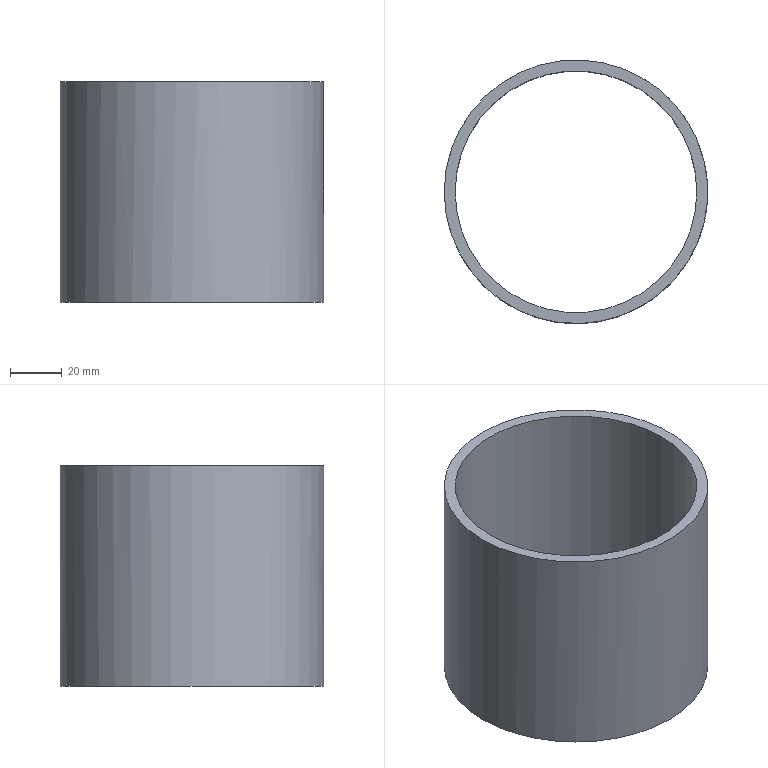Part | NX | features solid 2 | 1 solid | 4 faces | box 101.6 x 101.6 x 85 mm | volume 109239 mm3 | plane 2 | cylinder 2 | commonest cylinder face diameters 93.2 x1 101.6 x1
STEP:
#1=CARTESIAN_POINT('',(-1468.4,570.,-15.));
#2=VERTEX_POINT('',#1);
#3=CARTESIAN_POINT('',(-1515.,570.,-15.));
#4=DIRECTION('',(0.,0.,-1.));
#5=DIRECTION('',(1.,0.,0.));
#6=AXIS2_PLACEMENT_3D('',#3,#4,#5);
#7=CIRCLE('',#6,46.6);
#8=EDGE_CURVE('',#2,#2,#7,.T.);
#9=ORIENTED_EDGE('',*,*,#8,.F.);
#10=EDGE_LOOP('',(#9));
#11=FACE_BOUND('',#10,.T.);
#12=CARTESIAN_POINT('',(-1464.2,570.,-15.));
#13=VERTEX_POINT('',#12);
#14=CARTESIAN_POINT('',(-1515.,570.,-15.));
#15=DIRECTION('',(0.,0.,-1.));
#16=DIRECTION('',(1.,0.,0.));
#17=AXIS2_PLACEMENT_3D('',#14,#15,#16);
#18=CIRCLE('',#17,50.8);
#19=EDGE_CURVE('',#13,#13,#18,.T.);
#20=ORIENTED_EDGE('',*,*,#19,.T.);
#21=EDGE_LOOP('',(#20));
#22=FACE_BOUND('',#21,.T.);
#23=CARTESIAN_POINT('',(-1515.,570.,-15.));
#24=DIRECTION('',(0.,0.,-1.));
#25=DIRECTION('',(-1.,0.,0.));
#26=AXIS2_PLACEMENT_3D('',#23,#24,#25);
#27=PLANE('',#26);
#28=ADVANCED_FACE('',(#11,#22),#27,.T.);
#29=CARTESIAN_POINT('',(-1561.6,570.,70.));
#30=VERTEX_POINT('',#29);
#31=CARTESIAN_POINT('',(-1515.,570.,70.));
#32=DIRECTION('',(0.,0.,1.));
#33=DIRECTION('',(-1.,0.,0.));
#34=AXIS2_PLACEMENT_3D('',#31,#32,#33);
#35=CIRCLE('',#34,46.6);
#36=EDGE_CURVE('',#30,#30,#35,.T.);
#37=ORIENTED_EDGE('',*,*,#36,.F.);
#38=EDGE_LOOP('',(#37));
#39=FACE_BOUND('',#38,.T.);
#40=CARTESIAN_POINT('',(-1565.8,570.,70.));
#41=VERTEX_POINT('',#40);
#42=CARTESIAN_POINT('',(-1515.,570.,70.));
#43=DIRECTION('',(0.,0.,1.));
#44=DIRECTION('',(-1.,0.,0.));
#45=AXIS2_PLACEMENT_3D('',#42,#43,#44);
#46=CIRCLE('',#45,50.8);
#47=EDGE_CURVE('',#41,#41,#46,.T.);
#48=ORIENTED_EDGE('',*,*,#47,.T.);
#49=EDGE_LOOP('',(#48));
#50=FACE_BOUND('',#49,.T.);
#51=CARTESIAN_POINT('',(-1515.,570.,70.));
#52=DIRECTION('',(0.,0.,1.));
#53=DIRECTION('',(1.,0.,0.));
#54=AXIS2_PLACEMENT_3D('',#51,#52,#53);
#55=PLANE('',#54);
#56=ADVANCED_FACE('',(#39,#50),#55,.T.);
#57=ORIENTED_EDGE('',*,*,#19,.F.);
#58=EDGE_LOOP('',(#57));
#59=FACE_BOUND('',#58,.T.);
#60=ORIENTED_EDGE('',*,*,#47,.F.);
#61=EDGE_LOOP('',(#60));
#62=FACE_BOUND('',#61,.T.);
#63=CARTESIAN_POINT('',(-1515.,570.,70.));
#64=DIRECTION('',(0.,0.,-1.));
#65=DIRECTION('',(-1.,0.,0.));
#66=AXIS2_PLACEMENT_3D('',#63,#64,#65);
#67=CYLINDRICAL_SURFACE('',#66,50.8);
#68=ADVANCED_FACE('',(#59,#62),#67,.T.);
#69=ORIENTED_EDGE('',*,*,#8,.T.);
#70=EDGE_LOOP('',(#69));
#71=FACE_BOUND('',#70,.T.);
#72=ORIENTED_EDGE('',*,*,#36,.T.);
#73=EDGE_LOOP('',(#72));
#74=FACE_BOUND('',#73,.T.);
#75=CARTESIAN_POINT('',(-1515.,570.,70.));
#76=DIRECTION('',(0.,0.,-1.));
#77=DIRECTION('',(-1.,0.,0.));
#78=AXIS2_PLACEMENT_3D('',#75,#76,#77);
#79=CYLINDRICAL_SURFACE('',#78,46.6);
#80=ADVANCED_FACE('',(#71,#74),#79,.F.);
#81=CLOSED_SHELL('',(#28,#56,#68,#80));
#82=MANIFOLD_SOLID_BREP('',#81);
#83=(LENGTH_UNIT()NAMED_UNIT(*)SI_UNIT(.MILLI.,.METRE.));
#84=UNCERTAINTY_MEASURE_WITH_UNIT(LENGTH_MEASURE(0.00001),#83,'','');
#85=(NAMED_UNIT(*)PLANE_ANGLE_UNIT()SI_UNIT($,.RADIAN.));
#86=(NAMED_UNIT(*)SI_UNIT($,.STERADIAN.)SOLID_ANGLE_UNIT());
#87=(GEOMETRIC_REPRESENTATION_CONTEXT(3)GLOBAL_UNCERTAINTY_ASSIGNED_CONTEXT((#84))GLOBAL_UNIT_ASSIGNED_CONTEXT((#83,#85,#86))REPRESENTATION_CONTEXT('',''));
#88=ADVANCED_BREP_SHAPE_REPRESENTATION('',(#82),#87);